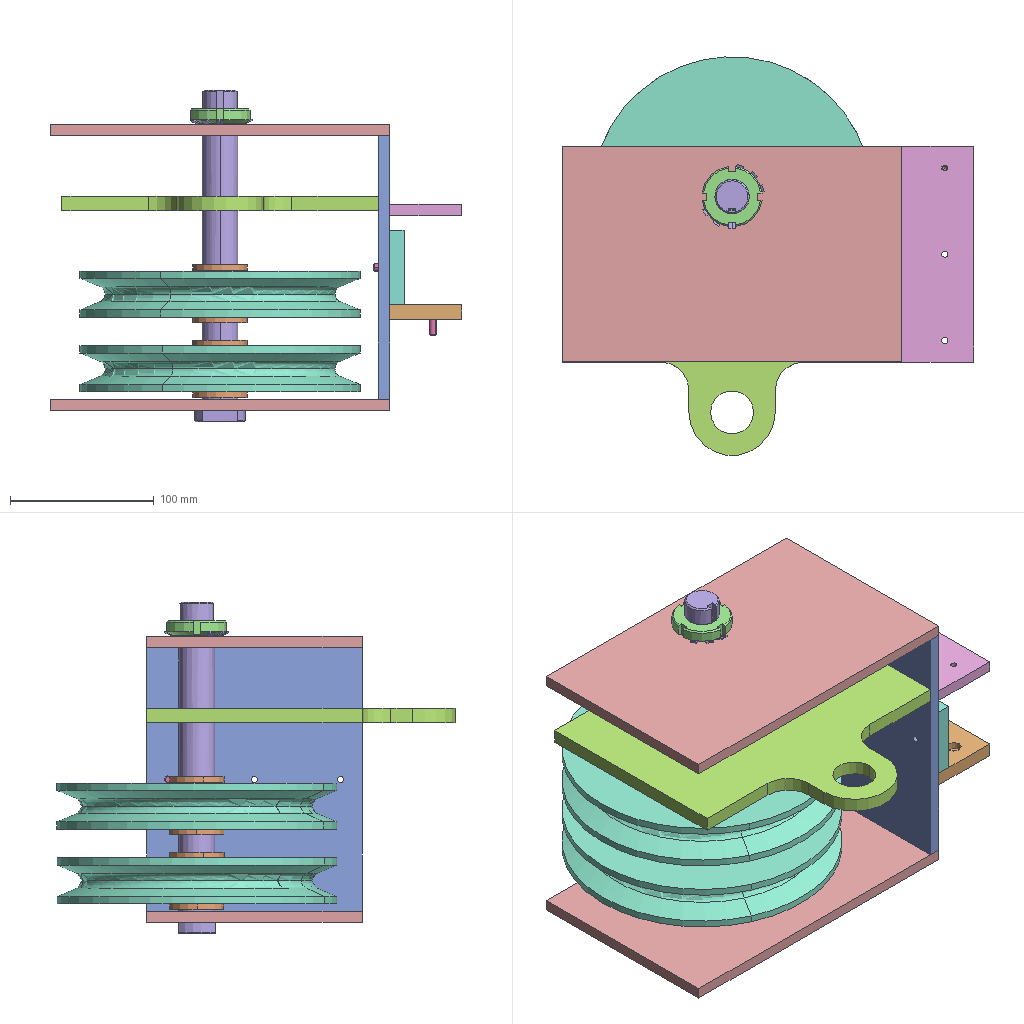Assembly | SolidWorks | 15 different items | 23 placed | box 286 x 277 x 231 mm
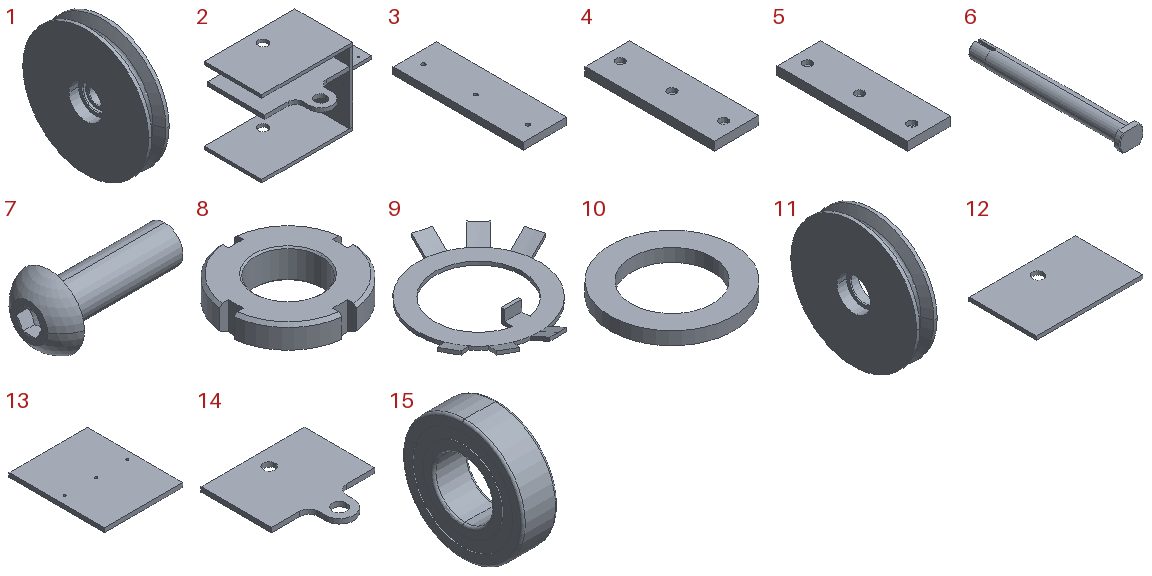Parts list (item | name | quantity | parent item | size | volume | features):
1 | (subassembly) | x2 | - | 32 x 195 x 195 mm | 764885 mm3 | -
2 | (subassembly) | x1 | - | 286 x 215 x 199 mm | 1192358 mm3 | -
3 | - | x1 | in 2 | 50 x 150 x 8 mm | 59667 mm3 | features Chamfer 1, Extrusion 1, HoleWzd 1
4 | - | x1 | - | 52 x 150 x 10 mm | 76527 mm3 | features Chamfer 1, Extrusion 1, HoleWzd 1
5 | - | x1 | - | 50 x 150 x 10 mm | 73527 mm3 | features Chamfer 1, Extrusion 1, HoleWzd 1
6 | - | x1 | - | 36 x 231 x 26 mm | 114684 mm3 | features Chamfer 2, Fillet 2, ICE 2, Revolution 1
7 | - | x2 | - | 18.75 x 9.5 x 9.5 mm | 431.838 mm3 | features RevCut 2, Revolution 2, Cut 1, LPattern 1, RefAxis 1
8 | - | x1 | - | 41.701 x 41.701 x 10 mm | 8727 mm3 | features Chamfer 3, CirPattern 1, Cut 1, Extrusion 1
9 | - | x1 | - | 42.805 x 44.602 x 4 mm | 623.641 mm3 | features Boss 1, Cut 1, Revolution 1
10 | - | x4 | - | 38 x 38 x 4 mm | 2573 mm3 | features Extrusion 1
11 | - | x2 | in 1 | 32 x 195 x 195 mm | 746203 mm3 | features ICE 2, MirrorPattern 1, Revolution 1
12 | - | x2 | in 2 | 236 x 150 x 8 mm | 279273 mm3 | features Extrusion 1, HoleWzd 1
13 | - | x1 | in 2 | 150 x 183 x 8 mm | 219267 mm3 | features Extrusion 1, HoleWzd 1
14 | - | x1 | in 2 | 220 x 215 x 10 mm | 354877 mm3 | features Extrusion 1, Fillet 1
15 | - | x2 | in 1 | 15 x 52 x 52 mm | 18682 mm3 | features Revolution 3, CirPattern 1, RefAxis 1
Mates (type | each side: item.copy, entity, surface, feature):
In the top assembly
Concentric | 12.1 face cylinder Ø25.0 (25) Diameter Hole1 | 6.1 face cylinder Revolve1
Coincident | 12.2 face plane Boss-Extrude1 | 6.1 face plane Revolve1
Parallel | 12.2 face plane Boss-Extrude1 | 6.1 face plane Cut-Extrude1
Concentric | 6.1 face cylinder Revolve1 | assembly face
Coincident | 15.1 face plane Revolve1 | 10.1 face plane Extrude1
Concentric | 10.2 face cylinder Extrude1 | 11.1 face cylinder Revolve1
Coincident | 11.1 face plane Revolve1 | 10.2 face plane Extrude1
Concentric | 6.1 face cylinder Revolve1 | 9.1 face cylinder Cut-Extrude2
Parallel | 9.1 face plane Cut-Extrude2 | 6.1 face plane Cut-Extrude2
Coincident | 12.1 face plane Boss-Extrude1 | 9.1 face plane Boss-Revolve1
Concentric | 6.1 face cylinder Revolve1 | 8.1 face cylinder Boss-Extrude1
Parallel | 12.1 face plane Boss-Extrude1 | 8.1 face plane CirPattern1
Coincident | 8.1 face plane Boss-Extrude1 | 9.1 face plane Boss-Revolve1
Concentric | 11.1 face cylinder Revolve1 | 10.1 face cylinder Extrude1
Concentric | 11.2 face cylinder Revolve1 | 10.3 face cylinder Extrude1
Coincident | 15.2 face plane Revolve1 | 10.4 face plane Extrude1
Concentric | 11.2 face cylinder Revolve1 | 10.4 face cylinder Extrude1
DistanceDim | 11.2 face plane Revolve1 | 10.3 face plane Extrude1
Concentric | 6.1 face cylinder Revolve1 | 11.2 face cylinder Revolve1
DistanceDim | 12.2 face plane Boss-Extrude1 | 10.1 face plane Extrude1
Coincident | 13.1 face plane Boss-Extrude1 | 4.1 face plane Boss-Extrude1 | 2 times
Concentric | 13.1 face cylinder M5 Tapped Hole1 | 4.1 face cylinder Hole1
Coincident | assembly face | 5.1 face plane Boss-Extrude1 | 2 times
Concentric | assembly face | 5.1 face cylinder Hole1
Concentric | 5.1 face cylinder Hole1 | 7.1 face cylinder Revolve1
Coincident | 5.1 face plane Hole1 | 7.1 face plane Revolve1
Concentric | 4.1 face cylinder Hole1 | 7.2 face cylinder Revolve1
Coincident | 4.1 face plane Hole1 | 7.2 face plane Revolve1
In subassembly 2
Coincident | 12.3 face plane Boss-Extrude1 | 2.1 plane
Coincident | 12.3 plane | 2.1 plane
Coincident | 12.3 face plane Boss-Extrude1 | 12.4 face plane Boss-Extrude1 | 2 times
Symmetric | 12.3 face plane Boss-Extrude1 | 12.4 face plane Boss-Extrude1 | 2.1 plane
DistanceDim | 12.3 face plane Boss-Extrude1 | 12.4 face plane Boss-Extrude1
Coincident | 12.3 face plane Boss-Extrude1 | 13.2 face plane Boss-Extrude1 | 3 times
Coincident | 13.2 face plane Boss-Extrude1 | 3.1 face plane Boss-Extrude1 | 2 times
Coincident | 13.2 face plane Boss-Extrude1 | 14.1 face plane Boss-Extrude1 | 2 times
DistanceDim | 14.1 face plane Boss-Extrude1 | 12.3 face plane Boss-Extrude1
In subassembly 1
Concentric | 11.3 face cylinder Cut-Extrude2 | 15.3 face cylinder Revolve1
Coincident | 11.3 face plane Cut-Extrude2 | 15.3 face plane Revolve1